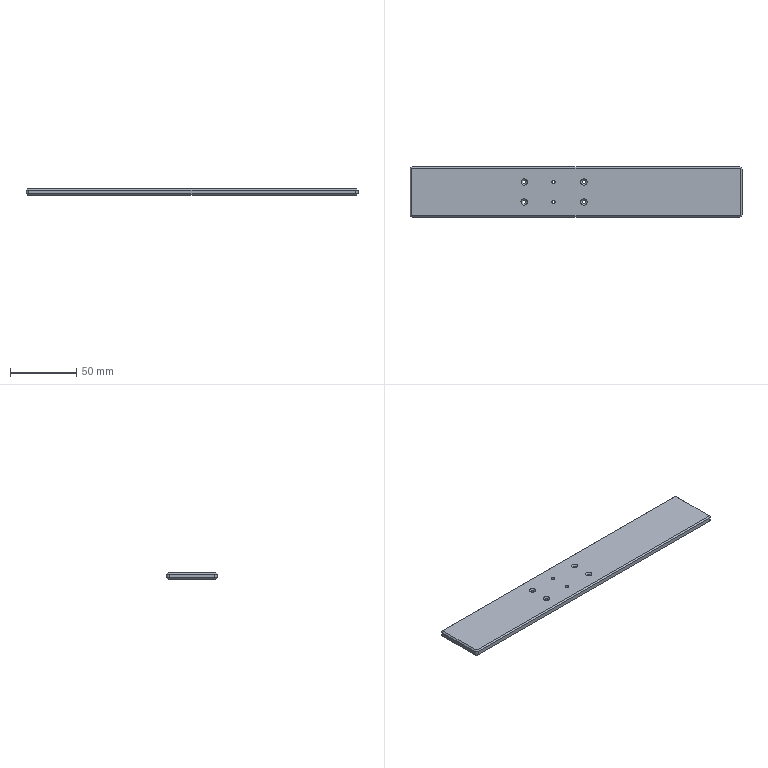NC program | NX | posted with a generic post | part box 250 x 38 x 5 mm
Lines 65 to 892 of 15324:
(ZLEVEL_PROFILE_COPY_COPY_1_COPY_COPY_1_COPY , TOOL : D2)
N128 T08 M6
N130 G54
N132 G17 G0 G90 X-39.808 Y-6.39 S7000 M3
N134 G43 Z35. H8
N136 Z6.5
N138 G94 G1 X-39.937 Y-6.474 Z6.492 F1000.
N140 X-40.219 Y-6.833 Z6.468
N142 X-40.369 Y-7.263 Z6.444
N144 X-40.372 Y-7.72 Z6.42
N146 X-40.227 Y-8.152 Z6.396
N148 X-40.037 Y-8.425 Z6.379
N150 X-39.786 Y-8.646 Z6.361
N152 X-39.49 Y-8.8 Z6.344
N154 X-39.166 Y-8.88 Z6.326
N156 X-38.834 Z6.309
N158 X-38.48 Y-8.789 Z6.29
N160 X-38.162 Y-8.609 Z6.271
N162 X-37.903 Y-8.352 Z6.252
N164 X-37.731 Y-8.067 Z6.234
N166 X-37.616 Y-7.621 Z6.21
N168 X-37.652 Y-7.163 Z6.186
N170 X-37.836 Y-6.741 Z6.162
N172 X-38.148 Y-6.403 Z6.138
N174 X-38.433 Y-6.231 Z6.12
N176 X-38.827 Y-6.121 Z6.099
N178 X-39.235 Y-6.13 Z6.077
N180 X-39.554 Y-6.226 Z6.06
N182 X-39.937 Y-6.474 Z6.036
N184 X-40.219 Y-6.833 Z6.012
N186 X-40.369 Y-7.263 Z5.988
N188 X-40.372 Y-7.72 Z5.964
N190 X-40.227 Y-8.152 Z5.94
N192 X-40.037 Y-8.425 Z5.923
N194 X-39.786 Y-8.646 Z5.905
N196 X-39.49 Y-8.8 Z5.888
N198 X-39.166 Y-8.88 Z5.871
N200 X-38.834 Z5.853
N202 X-38.48 Y-8.789 Z5.834
N204 X-38.162 Y-8.609 Z5.815
N206 X-37.903 Y-8.352 Z5.796
N208 X-37.731 Y-8.067 Z5.778
N210 X-37.616 Y-7.621 Z5.754
N212 X-37.652 Y-7.163 Z5.73
N214 X-37.836 Y-6.741 Z5.706
N216 X-38.148 Y-6.403 Z5.682
N218 X-38.433 Y-6.231 Z5.664
N220 X-38.827 Y-6.121 Z5.643
N222 X-39.235 Y-6.13 Z5.622
N224 X-39.554 Y-6.226 Z5.604
N226 X-39.937 Y-6.474 Z5.58
N228 X-40.219 Y-6.833 Z5.556
N230 X-40.369 Y-7.263 Z5.532
N232 X-40.372 Y-7.72 Z5.508
N234 X-40.227 Y-8.152 Z5.485
N236 X-40.037 Y-8.425 Z5.467
N238 X-39.786 Y-8.646 Z5.45
N240 X-39.49 Y-8.8 Z5.432
N242 X-39.166 Y-8.88 Z5.415
N244 X-38.834 Z5.397
N246 X-38.48 Y-8.789 Z5.378
N248 X-38.162 Y-8.609 Z5.359
N250 X-37.903 Y-8.352 Z5.34
N252 X-37.731 Y-8.067 Z5.322
N254 X-37.616 Y-7.621 Z5.298
N256 X-37.652 Y-7.163 Z5.274
N258 X-37.836 Y-6.741 Z5.25
N260 X-38.148 Y-6.403 Z5.226
N262 X-38.433 Y-6.231 Z5.208
N264 X-38.827 Y-6.121 Z5.187
N266 X-39.235 Y-6.13 Z5.166
N268 X-39.554 Y-6.226 Z5.148
N270 X-39.937 Y-6.474 Z5.124
N272 X-40.219 Y-6.833 Z5.1
N274 X-40.369 Y-7.263 Z5.076
N276 X-40.372 Y-7.72 Z5.053
N278 X-40.227 Y-8.152 Z5.029
N280 X-40.037 Y-8.425 Z5.011
N282 X-39.786 Y-8.646 Z4.994
N284 X-39.49 Y-8.8 Z4.976
N286 X-39.166 Y-8.88 Z4.959
N288 X-39. Z4.95
N290 G3 X-37.621 Y-7.5 R1.379
N292 X-39. Y-8.88 R-1.379
N294 G1 X-38.905 Y-8.875 Z4.948
N296 X-38.81 Y-8.863 Z4.947
N298 X-38.717 Y-8.845 Z4.945
N300 X-38.625 Y-8.821 Z4.943
N302 X-38.535 Y-8.79 Z4.942
N304 X-38.447 Y-8.753 Z4.94
N306 X-38.363 Y-8.71 Z4.938
N308 X-38.282 Y-8.662 Z4.937
N310 X-38.204 Y-8.608 Z4.935
N312 X-38.13 Y-8.549 Z4.933
N314 X-38.061 Y-8.485 Z4.932
N316 X-37.996 Y-8.417 Z4.93
N318 X-37.937 Y-8.344 Z4.928
N320 X-37.882 Y-8.268 Z4.927
N322 X-37.833 Y-8.188 Z4.925
N324 X-37.79 Y-8.105 Z4.923
N326 X-37.752 Y-8.019 Z4.922
N328 X-37.721 Y-7.931 Z4.92
N330 X-37.696 Y-7.841 Z4.918
N332 X-37.677 Y-7.75 Z4.917
N334 X-37.665 Y-7.657 Z4.915
N336 X-37.659 Y-7.564 Z4.913
N338 Y-7.472 Z4.912
N340 X-37.666 Y-7.379 Z4.91
N342 X-37.679 Y-7.288 Z4.908
N344 X-37.699 Y-7.197 Z4.907
N346 X-37.724 Y-7.108 Z4.905
N348 X-37.756 Y-7.021 Z4.903
N350 X-37.794 Y-6.937 Z4.902
N352 X-37.837 Y-6.856 Z4.9
N354 G3 X-39. Y-8.83 R-1.329
N356 G1 X-38.905 Y-8.824 Z4.898
N358 X-38.81 Y-8.813 Z4.897
N360 X-38.717 Y-8.794 Z4.895
N362 X-38.625 Y-8.769 Z4.893
N364 X-38.536 Y-8.737 Z4.892
N366 X-38.449 Y-8.699 Z4.89
N368 X-38.365 Y-8.655 Z4.888
N370 X-38.285 Y-8.605 Z4.887
N372 X-38.208 Y-8.549 Z4.885
N374 X-38.136 Y-8.489 Z4.883
N376 X-38.069 Y-8.423 Z4.882
N378 X-38.006 Y-8.353 Z4.88
N380 X-37.949 Y-8.278 Z4.878
N382 X-37.897 Y-8.2 Z4.877
N384 X-37.851 Y-8.118 Z4.875
N386 X-37.811 Y-8.033 Z4.873
N388 X-37.778 Y-7.946 Z4.872
N390 X-37.75 Y-7.857 Z4.87
N392 X-37.73 Y-7.766 Z4.868
N394 X-37.716 Y-7.674 Z4.867
N396 X-37.708 Y-7.581 Z4.865
N398 X-37.707 Y-7.488 Z4.863
N400 X-37.713 Y-7.396 Z4.862
N402 X-37.726 Y-7.304 Z4.86
N404 X-37.745 Y-7.213 Z4.858
N406 X-37.77 Y-7.124 Z4.857
N408 X-37.802 Y-7.038 Z4.855
N410 X-37.839 Y-6.953 Z4.853
N412 X-37.883 Y-6.872 Z4.852
N414 X-37.932 Y-6.795 Z4.85
N416 G3 X-39. Y-8.78 R-1.279
N418 G1 X-38.905 Y-8.774 Z4.848
N420 X-38.81 Y-8.762 Z4.847
N422 X-38.717 Y-8.743 Z4.845
N424 X-38.626 Y-8.717 Z4.843
N426 X-38.537 Y-8.684 Z4.842
N428 X-38.45 Y-8.644 Z4.84
N430 X-38.368 Y-8.599 Z4.838
N432 X-38.288 Y-8.547 Z4.837
N434 X-38.213 Y-8.49 Z4.835
N436 X-38.143 Y-8.427 Z4.833
N438 X-38.077 Y-8.36 Z4.832
N440 X-38.017 Y-8.287 Z4.83
N442 X-37.962 Y-8.211 Z4.828
N444 X-37.914 Y-8.131 Z4.827
N446 X-37.871 Y-8.047 Z4.825
N448 X-37.835 Y-7.961 Z4.823
N450 X-37.806 Y-7.872 Z4.822
N452 X-37.783 Y-7.782 Z4.82
N454 X-37.767 Y-7.69 Z4.818
N456 X-37.758 Y-7.597 Z4.817
N458 X-37.756 Y-7.505 Z4.815
N460 X-37.76 Y-7.412 Z4.813
N462 X-37.772 Y-7.32 Z4.812
N464 X-37.79 Y-7.229 Z4.81
N466 X-37.816 Y-7.14 Z4.808
N468 X-37.847 Y-7.054 Z4.807
N470 X-37.885 Y-6.97 Z4.805
N472 X-37.929 Y-6.889 Z4.803
N474 X-37.979 Y-6.812 Z4.802
N476 X-38.035 Y-6.738 Z4.8
N478 G3 X-39. Y-8.73 R-1.229
N480 G1 X-38.905 Y-8.724 Z4.798
N482 X-38.81 Y-8.711 Z4.797
N484 X-38.717 Y-8.691 Z4.795
N486 X-38.626 Y-8.664 Z4.793
N488 X-38.538 Y-8.63 Z4.792
N490 X-38.452 Y-8.589 Z4.79
N492 X-38.37 Y-8.542 Z4.788
N494 X-38.292 Y-8.489 Z4.787
N496 X-38.219 Y-8.43 Z4.785
N498 X-38.15 Y-8.365 Z4.783
N500 X-38.087 Y-8.296 Z4.782
N502 X-38.029 Y-8.221 Z4.78
N504 X-37.978 Y-8.143 Z4.778
N506 X-37.932 Y-8.061 Z4.777
N508 X-37.893 Y-7.976 Z4.775
N510 X-37.861 Y-7.888 Z4.773
N512 X-37.836 Y-7.798 Z4.772
N514 X-37.818 Y-7.706 Z4.77
N516 X-37.808 Y-7.614 Z4.768
N518 X-37.804 Y-7.521 Z4.767
N520 X-37.808 Y-7.428 Z4.765
N522 X-37.818 Y-7.336 Z4.763
N524 X-37.836 Y-7.246 Z4.762
N526 X-37.861 Y-7.156 Z4.76
N528 X-37.893 Y-7.07 Z4.758
N530 X-37.931 Y-6.986 Z4.757
N532 X-37.976 Y-6.905 Z4.755
N534 X-38.026 Y-6.829 Z4.753
N536 X-38.082 Y-6.756 Z4.752
N538 X-38.144 Y-6.688 Z4.75
N540 G3 X-39. Y-8.68 R-1.179
N542 G1 X-38.905 Y-8.674 Z4.748
N544 X-38.81 Y-8.661 Z4.747
N546 X-38.718 Y-8.64 Z4.745
N548 X-38.627 Y-8.612 Z4.743
N550 X-38.539 Y-8.577 Z4.742
N552 X-38.454 Y-8.534 Z4.74
N554 X-38.373 Y-8.485 Z4.738
N556 X-38.296 Y-8.43 Z4.737
N558 X-38.225 Y-8.369 Z4.735
N560 X-38.158 Y-8.302 Z4.733
N562 X-38.097 Y-8.231 Z4.732
N564 X-38.043 Y-8.154 Z4.73
N566 X-37.994 Y-8.074 Z4.728
N568 X-37.953 Y-7.99 Z4.727
N570 X-37.918 Y-7.903 Z4.725
N572 X-37.891 Y-7.814 Z4.723
N574 X-37.871 Y-7.723 Z4.722
N576 X-37.858 Y-7.63 Z4.72
N578 X-37.853 Y-7.538 Z4.718
N580 X-37.855 Y-7.445 Z4.717
N582 X-37.865 Y-7.353 Z4.715
N584 X-37.882 Y-7.262 Z4.713
N586 X-37.907 Y-7.173 Z4.712
N588 X-37.938 Y-7.086 Z4.71
N590 X-37.977 Y-7.002 Z4.708
N592 X-38.022 Y-6.922 Z4.707
N594 X-38.073 Y-6.846 Z4.705
N596 X-38.131 Y-6.774 Z4.703
N598 X-38.193 Y-6.707 Z4.702
N600 X-38.261 Y-6.646 Z4.7
N602 G3 X-39. Y-8.63 R-1.129
N604 G1 X-38.905 Y-8.624 Z4.698
N606 X-38.811 Y-8.61 Z4.697
N608 X-38.718 Y-8.589 Z4.695
N610 X-38.628 Y-8.559 Z4.693
N612 X-38.54 Y-8.523 Z4.692
N614 X-38.456 Y-8.479 Z4.69
N616 X-38.377 Y-8.428 Z4.688
N618 X-38.301 Y-8.371 Z4.687
N620 X-38.232 Y-8.307 Z4.685
N622 X-38.167 Y-8.238 Z4.683
N624 X-38.109 Y-8.165 Z4.682
N626 X-38.058 Y-8.086 Z4.68
N628 X-38.013 Y-8.004 Z4.678
N630 X-37.976 Y-7.918 Z4.677
N632 X-37.946 Y-7.829 Z4.675
N634 X-37.923 Y-7.739 Z4.673
N636 X-37.909 Y-7.647 Z4.672
N638 X-37.902 Y-7.554 Z4.67
N640 X-37.903 Y-7.461 Z4.668
N642 X-37.912 Y-7.369 Z4.667
N644 X-37.928 Y-7.278 Z4.665
N646 X-37.952 Y-7.189 Z4.663
N648 X-37.984 Y-7.102 Z4.662
N650 X-38.023 Y-7.018 Z4.66
N652 X-38.068 Y-6.938 Z4.658
N654 X-38.121 Y-6.863 Z4.657
N656 X-38.179 Y-6.792 Z4.655
N658 X-38.243 Y-6.726 Z4.653
N660 X-38.312 Y-6.666 Z4.652
N662 X-38.386 Y-6.612 Z4.65
N664 G3 X-39. Y-8.58 R-1.079
N666 G1 X-38.905 Y-8.574 Z4.648
N668 X-38.811 Y-8.559 Z4.647
N670 X-38.718 Y-8.537 Z4.645
N672 X-38.628 Y-8.506 Z4.643
N674 X-38.542 Y-8.468 Z4.642
N676 X-38.459 Y-8.422 Z4.64
N678 X-38.38 Y-8.37 Z4.638
N680 X-38.307 Y-8.31 Z4.637
N682 X-38.239 Y-8.245 Z4.635
N684 X-38.178 Y-8.173 Z4.633
N686 X-38.123 Y-8.097 Z4.632
N688 X-38.075 Y-8.017 Z4.63
N690 X-38.035 Y-7.932 Z4.628
N692 X-38.002 Y-7.845 Z4.627
N694 X-37.977 Y-7.755 Z4.625
N696 X-37.96 Y-7.663 Z4.623
N698 X-37.951 Y-7.571 Z4.622
N700 Y-7.478 Z4.62
N702 X-37.958 Y-7.385 Z4.618
N704 X-37.974 Y-7.294 Z4.617
N706 X-37.998 Y-7.205 Z4.615
N708 X-38.03 Y-7.118 Z4.613
N710 X-38.069 Y-7.035 Z4.612
N712 X-38.115 Y-6.955 Z4.61
N714 X-38.168 Y-6.88 Z4.608
N716 X-38.227 Y-6.81 Z4.607
N718 X-38.292 Y-6.746 Z4.605
N720 X-38.363 Y-6.687 Z4.603
N722 X-38.438 Y-6.636 Z4.602
N724 X-38.517 Y-6.591 Z4.6
N726 G3 X-39. Y-8.53 R-1.029
N728 G1 X-38.905 Y-8.523 Z4.598
N730 X-38.811 Y-8.509 Z4.597
N732 X-38.706 Y-8.481 Z4.595
N734 X-38.629 Y-8.453 Z4.593
N736 X-38.529 Y-8.406 Z4.591
N738 X-38.461 Y-8.366 Z4.59
N740 X-38.372 Y-8.301 Z4.588
N742 X-38.313 Y-8.249 Z4.587
N744 X-38.238 Y-8.169 Z4.585
N746 X-38.19 Y-8.108 Z4.583
N748 X-38.13 Y-8.015 Z4.581
N750 X-38.094 Y-7.946 Z4.58
N752 X-38.053 Y-7.845 Z4.578
N754 X-38.031 Y-7.771 Z4.577
N756 X-38.009 Y-7.664 Z4.575
N758 X-38.001 Y-7.587 Z4.573
N760 X-37.999 Y-7.478 Z4.571
N762 X-38.005 Y-7.402 Z4.57
N764 X-38.024 Y-7.295 Z4.568
N766 X-38.044 Y-7.221 Z4.567
N768 X-38.081 Y-7.12 Z4.565
N770 X-38.115 Y-7.051 Z4.563
N772 X-38.17 Y-6.958 Z4.561
N774 X-38.215 Y-6.897 Z4.56
N776 X-38.287 Y-6.817 Z4.558
N778 X-38.342 Y-6.765 Z4.557
N780 X-38.427 Y-6.7 Z4.555
N782 X-38.491 Y-6.659 Z4.553
N784 X-38.571 Y-6.617 Z4.552
N786 X-38.656 Y-6.583 Z4.55
N788 G3 X-39. Y-8.48 R-0.979
N790 G1 X-38.905 Y-8.473 Z4.548
N792 X-38.811 Y-8.458 Z4.547
N794 X-38.706 Y-8.429 Z4.545
N796 X-38.63 Y-8.4 Z4.543
N798 X-38.532 Y-8.35 Z4.541
N800 X-38.465 Y-8.308 Z4.54
N802 X-38.378 Y-8.241 Z4.538
N804 X-38.321 Y-8.187 Z4.537
N806 X-38.248 Y-8.104 Z4.535
N808 X-38.203 Y-8.04 Z4.533
N810 X-38.149 Y-7.945 Z4.531
N812 X-38.117 Y-7.875 Z4.53
N814 X-38.082 Y-7.771 Z4.528
N816 X-38.064 Y-7.696 Z4.527
N818 X-38.05 Y-7.588 Z4.525
N820 X-38.047 Y-7.511 Z4.523
N822 X-38.054 Y-7.402 Z4.521
N824 X-38.067 Y-7.326 Z4.52
N826 X-38.094 Y-7.222 Z4.518
N828 X-38.121 Y-7.15 Z4.517
N830 X-38.168 Y-7.053 Z4.515
N832 X-38.208 Y-6.988 Z4.513
N834 X-38.273 Y-6.903 Z4.511
N836 X-38.325 Y-6.847 Z4.51
N838 X-38.405 Y-6.776 Z4.508
N840 X-38.466 Y-6.731 Z4.507
N842 X-38.558 Y-6.677 Z4.505
N844 X-38.626 Y-6.645 Z4.503
N846 X-38.712 Y-6.615 Z4.502
N848 X-38.8 Y-6.592 Z4.5
N850 G3 X-39. Y-8.43 R-0.929
N852 G1 X-38.88 Y-8.42 Z4.498
N854 X-38.811 Y-8.407 Z4.497
N856 X-38.703 Y-8.375 Z4.495
N858 X-38.631 Y-8.346 Z4.493
N860 X-38.533 Y-8.294 Z4.491
N862 X-38.468 Y-8.25 Z4.49
N864 X-38.384 Y-8.18 Z4.488
N866 X-38.329 Y-8.124 Z4.487
N868 X-38.261 Y-8.038 Z4.485
N870 X-38.219 Y-7.972 Z4.483
N872 X-38.17 Y-7.874 Z4.481
N874 X-38.142 Y-7.802 Z4.48
N876 X-38.114 Y-7.696 Z4.478
N878 X-38.102 Y-7.62 Z4.477
N880 X-38.096 Y-7.511 Z4.475
N882 X-38.1 Y-7.434 Z4.473
N884 X-38.116 Y-7.327 Z4.471
N886 X-38.135 Y-7.253 Z4.47
N888 X-38.173 Y-7.152 Z4.468
N890 X-38.207 Y-7.083 Z4.467
N892 X-38.264 Y-6.992 Z4.465
N894 X-38.311 Y-6.932 Z4.463
N896 X-38.385 Y-6.855 Z4.461
N898 X-38.443 Y-6.806 Z4.46
N900 X-38.532 Y-6.746 Z4.458
N902 X-38.598 Y-6.71 Z4.457
N904 X-38.696 Y-6.67 Z4.455
N906 X-38.769 Y-6.648 Z4.453
N908 X-38.857 Y-6.63 Z4.452
N910 X-38.947 Y-6.622 Z4.45
N912 G3 X-39. Y-8.38 R-0.879
N914 G1 X-38.88 Y-8.369 Z4.448
N916 X-38.811 Y-8.356 Z4.447
N918 X-38.704 Y-8.322 Z4.445
N920 X-38.633 Y-8.292 Z4.443
N922 X-38.536 Y-8.237 Z4.441
N924 X-38.473 Y-8.191 Z4.44
N926 X-38.391 Y-8.118 Z4.438
N928 X-38.339 Y-8.06 Z4.437
N930 X-38.275 Y-7.97 Z4.435
N932 X-38.237 Y-7.902 Z4.433
N934 X-38.194 Y-7.802 Z4.431
N936 X-38.171 Y-7.728 Z4.43
N938 X-38.151 Y-7.621 Z4.428
N940 X-38.145 Y-7.544 Z4.427
N942 X-38.148 Y-7.435 Z4.425
N944 X-38.159 Y-7.359 Z4.423
N946 X-38.185 Y-7.254 Z4.421
N948 X-38.212 Y-7.182 Z4.42
N950 X-38.26 Y-7.086 Z4.418
N952 X-38.302 Y-7.022 Z4.417
N954 X-38.37 Y-6.939 Z4.415
N956 X-38.424 Y-6.885 Z4.413
N958 X-38.507 Y-6.819 Z4.411
N960 X-38.571 Y-6.778 Z4.41
N962 X-38.667 Y-6.732 Z4.408
N964 X-38.738 Y-6.706 Z4.407
N966 X-38.841 Y-6.681 Z4.405
N968 X-38.915 Y-6.671 Z4.403
N970 X-39.005 Y-6.669 Z4.402
N972 X-39.095 Y-6.676 Z4.4
N974 G3 X-39. Y-8.33 R0.829
N976 G1 X-38.88 Y-8.319 Z4.398
N978 X-38.811 Y-8.304 Z4.397
N980 X-38.704 Y-8.269 Z4.395
N982 X-38.634 Y-8.237 Z4.393
N984 X-38.54 Y-8.18 Z4.391
N986 X-38.478 Y-8.132 Z4.39
N988 X-38.399 Y-8.055 Z4.388
N990 X-38.35 Y-7.994 Z4.387
N992 X-38.291 Y-7.901 Z4.385
N994 X-38.258 Y-7.831 Z4.383
N996 X-38.222 Y-7.728 Z4.381
N998 X-38.205 Y-7.652 Z4.38
N1000 X-38.194 Y-7.544 Z4.378
N1002 X-38.195 Y-7.467 Z4.377
N1004 X-38.208 Y-7.36 Z4.375
N1006 X-38.226 Y-7.285 Z4.373
N1008 X-38.264 Y-7.184 Z4.371
N1010 X-38.299 Y-7.116 Z4.37
N1012 X-38.358 Y-7.026 Z4.368
N1014 X-38.407 Y-6.968 Z4.367
N1016 X-38.485 Y-6.895 Z4.365
N1018 X-38.546 Y-6.85 Z4.363
N1020 X-38.639 Y-6.797 Z4.361
N1022 X-38.708 Y-6.767 Z4.36
N1024 X-38.81 Y-6.736 Z4.358
N1026 X-38.883 Y-6.723 Z4.357
N1028 X-38.989 Y-6.716 Z4.355
N1030 X-39.064 Y-6.72 Z4.353
N1032 X-39.152 Y-6.734 Z4.352
N1034 X-39.239 Y-6.758 Z4.35
N1036 G3 X-39. Y-8.28 R0.779
N1038 G1 X-38.879 Y-8.268 Z4.348
N1040 X-38.812 Y-8.253 Z4.347
N1042 X-38.705 Y-8.216 Z4.345
N1044 X-38.636 Y-8.182 Z4.343
N1046 X-38.544 Y-8.121 Z4.341
N1048 X-38.484 Y-8.071 Z4.34
N1050 X-38.409 Y-7.99 Z4.338
N1052 X-38.364 Y-7.927 Z4.337
N1054 X-38.311 Y-7.831 Z4.335
N1056 X-38.282 Y-7.759 Z4.333
N1058 X-38.255 Y-7.653 Z4.331
N1060 X-38.244 Y-7.576 Z4.33
N1062 X-38.243 Y-7.468 Z4.328
N1064 X-38.252 Y-7.391 Z4.327
N1066 X-38.277 Y-7.286 Z4.325
N1068 X-38.303 Y-7.214 Z4.323
N1070 X-38.353 Y-7.119 Z4.321
N1072 X-38.396 Y-7.056 Z4.32
N1074 X-38.467 Y-6.976 Z4.318
N1076 X-38.524 Y-6.925 Z4.317
N1078 X-38.612 Y-6.865 Z4.315
N1080 X-38.679 Y-6.83 Z4.313
N1082 X-38.779 Y-6.793 Z4.311
N1084 X-38.852 Y-6.776 Z4.31
N1086 X-38.957 Y-6.764 Z4.308
N1088 X-39.032 Y-6.765 Z4.307
N1090 X-39.136 Y-6.779 Z4.305
N1092 X-39.208 Y-6.797 Z4.303
N1094 X-39.292 Y-6.83 Z4.302
N1096 X-39.371 Y-6.872 Z4.3
N1098 G3 X-39. Y-8.23 R0.729
N1100 G1 X-38.879 Y-8.217 Z4.298
N1102 X-38.812 Y-8.201 Z4.297
N1104 X-38.707 Y-8.162 Z4.295
N1106 X-38.639 Y-8.126 Z4.293
N1108 X-38.548 Y-8.062 Z4.291
N1110 X-38.491 Y-8.009 Z4.29
N1112 X-38.421 Y-7.924 Z4.288
N1114 X-38.38 Y-7.858 Z4.287
N1116 X-38.334 Y-7.759 Z4.285
N1118 X-38.311 Y-7.685 Z4.283
N1120 X-38.293 Y-7.577 Z4.281
N1122 X-38.291 Y-7.5 Z4.28
N1124 X-38.301 Y-7.392 Z4.278
N1126 X-38.318 Y-7.317 Z4.277
N1128 X-38.355 Y-7.216 Z4.275
N1130 X-38.391 Y-7.149 Z4.273
N1132 X-38.453 Y-7.061 Z4.271
N1134 X-38.505 Y-7.005 Z4.27
N1136 X-38.588 Y-6.937 Z4.268
N1138 X-38.652 Y-6.897 Z4.267
N1140 X-38.748 Y-6.853 Z4.265
N1142 X-38.821 Y-6.831 Z4.263
N1144 X-38.925 Y-6.813 Z4.261
N1146 X-39. Y-6.811 Z4.26
N1148 X-39.105 Y-6.82 Z4.258
N1150 X-39.177 Y-6.837 Z4.257
N1152 X-39.276 Y-6.874 Z4.255
N1154 X-39.341 Y-6.909 Z4.253
N1156 X-39.414 Y-6.959 Z4.252
N1158 X-39.48 Y-7.019 Z4.25
N1160 G3 X-39. Y-8.18 R0.679
N1162 G1 X-38.879 Y-8.166 Z4.248
N1164 X-38.812 Y-8.15 Z4.247
N1166 X-38.708 Y-8.108 Z4.245
N1168 X-38.641 Y-8.069 Z4.243
N1170 X-38.554 Y-8.001 Z4.241
N1172 X-38.5 Y-7.945 Z4.24
N1174 X-38.436 Y-7.856 Z4.238
N1176 X-38.399 Y-7.788 Z4.237
N1178 X-38.362 Y-7.685 Z4.235
N1180 X-38.346 Y-7.609 Z4.233
N1182 X-38.339 Y-7.501 Z4.231
N1184 X-38.345 Y-7.424 Z4.23
N1186 X-38.368 Y-7.318 Z4.228
N1188 X-38.395 Y-7.247 Z4.227
N1190 X-38.446 Y-7.152 Z4.225
N1192 X-38.491 Y-7.091 Z4.223
N1194 X-38.566 Y-7.015 Z4.221
N1196 X-38.627 Y-6.968 Z4.22
N1198 X-38.72 Y-6.916 Z4.218
N1200 X-38.79 Y-6.889 Z4.217
N1202 X-38.893 Y-6.865 Z4.215
N1204 X-38.968 Y-6.858 Z4.213
N1206 X-39.073 Y-6.863 Z4.211
N1208 X-39.146 Y-6.877 Z4.21
N1210 X-39.245 Y-6.912 Z4.208
N1212 X-39.312 Y-6.945 Z4.207
N1214 X-39.397 Y-7.005 Z4.205
N1216 X-39.451 Y-7.056 Z4.203
N1218 X-39.507 Y-7.124 Z4.202
N1220 X-39.553 Y-7.2 Z4.2
N1222 G3 X-39. Y-8.13 R0.629
N1224 G1 X-38.876 Y-8.115 Z4.198
N1226 X-38.809 Y-8.096 Z4.196
N1228 X-38.704 Y-8.049 Z4.194
N1230 X-38.639 Y-8.007 Z4.193
N1232 X-38.554 Y-7.932 Z4.191
N1234 X-38.504 Y-7.87 Z4.189
N1236 X-38.447 Y-7.774 Z4.187
N1238 X-38.418 Y-7.7 Z4.186
N1240 X-38.394 Y-7.592 Z4.184
N1242 X-38.388 Y-7.513 Z4.182
N1244 X-38.398 Y-7.403 Z4.18
N1246 X-38.417 Y-7.327 Z4.179
N1248 X-38.46 Y-7.226 Z4.176
N1250 X-38.5 Y-7.16 Z4.175
N1252 X-38.571 Y-7.077 Z4.173
N1254 X-38.63 Y-7.026 Z4.171
N1256 X-38.723 Y-6.969 Z4.169
N1258 X-38.794 Y-6.939 Z4.168
N1260 X-38.898 Y-6.913 Z4.166
N1262 X-38.975 Y-6.907 Z4.164
N1264 X-39.081 Y-6.914 Z4.162
N1266 X-39.156 Y-6.931 Z4.161
N1268 X-39.255 Y-6.97 Z4.159
N1270 X-39.32 Y-7.008 Z4.157
N1272 X-39.402 Y-7.075 Z4.155
N1274 X-39.452 Y-7.131 Z4.154
N1276 X-39.502 Y-7.206 Z4.152
N1278 X-39.539 Y-7.288 Z4.15
N1280 G3 X-39. Y-8.08 R0.579
N1282 G1 X-38.879 Y-8.064 Z4.148
N1284 X-38.813 Y-8.044 Z4.146
N1286 X-38.711 Y-7.995 Z4.144
N1288 X-38.648 Y-7.951 Z4.142
N1290 X-38.57 Y-7.873 Z4.14
N1292 X-38.524 Y-7.81 Z4.138
N1294 X-38.475 Y-7.712 Z4.136
N1296 X-38.453 Y-7.637 Z4.135
N1298 X-38.439 Y-7.529 Z4.132
N1300 X-38.442 Y-7.452 Z4.131
N1302 X-38.464 Y-7.346 Z4.129
N1304 X-38.491 Y-7.275 Z4.127
N1306 X-38.546 Y-7.183 Z4.125
N1308 X-38.595 Y-7.124 Z4.123
N1310 X-38.676 Y-7.055 Z4.121
N1312 X-38.741 Y-7.016 Z4.119
N1314 X-38.839 Y-6.978 Z4.117
N1316 X-38.913 Y-6.962 Z4.115
N1318 X-39.018 Y-6.958 Z4.113
N1320 X-39.092 Y-6.967 Z4.112
N1322 X-39.192 Y-6.997 Z4.109
N1324 X-39.258 Y-7.029 Z4.108
N1326 X-39.343 Y-7.089 Z4.105
N1328 X-39.395 Y-7.141 Z4.104
N1330 X-39.447 Y-7.212 Z4.102
N1332 X-39.486 Y-7.291 Z4.1
N1334 G3 X-39. Y-8.03 R0.529
N1336 G1 X-38.881 Y-8.013 Z4.097
N1338 X-38.817 Y-7.992 Z4.096
N1340 X-38.719 Y-7.941 Z4.093
N1342 X-38.66 Y-7.895 Z4.092
N1344 X-38.587 Y-7.814 Z4.089
N1346 X-38.547 Y-7.75 Z4.088
N1348 X-38.508 Y-7.65 Z4.085
N1350 X-38.493 Y-7.576 Z4.083
N1352 X-38.49 Y-7.47 Z4.081
N1354 X-38.502 Y-7.395 Z4.079
N1356 X-38.537 Y-7.296 Z4.077
N1358 X-38.573 Y-7.231 Z4.075
N1360 X-38.64 Y-7.15 Z4.073
N1362 X-38.696 Y-7.102 Z4.071
N1364 X-38.786 Y-7.051 Z4.068
N1366 X-38.855 Y-7.026 Z4.067
N1368 X-38.956 Y-7.008 Z4.064
N1370 X-39.029 Y-7.009 Z4.063
N1372 X-39.129 Y-7.028 Z4.06
N1374 X-39.197 Y-7.053 Z4.058
N1376 X-39.283 Y-7.106 Z4.056
N1378 X-39.337 Y-7.153 Z4.054
N1380 X-39.391 Y-7.219 Z4.052
N1382 X-39.433 Y-7.294 Z4.05
N1384 G3 X-39. Y-7.98 R0.479
N1386 G1 X-38.885 Y-7.962 Z4.047
N1388 X-38.822 Y-7.94 Z4.045
N1390 X-38.729 Y-7.887 Z4.043
N1392 X-38.673 Y-7.839 Z4.041
N1394 X-38.608 Y-7.756 Z4.038
N1396 X-38.575 Y-7.69 Z4.036
N1398 X-38.546 Y-7.59 Z4.034
N1400 X-38.539 Y-7.517 Z4.032
N1402 X-38.549 Y-7.414 Z4.029
N1404 X-38.571 Y-7.344 Z4.027
N1406 X-38.618 Y-7.254 Z4.025
N1408 X-38.663 Y-7.198 Z4.023
N1410 X-38.741 Y-7.133 Z4.02
N1412 X-38.803 Y-7.098 Z4.018
N1414 X-38.898 Y-7.067 Z4.016
N1416 X-38.968 Y-7.058 Z4.014
N1418 X-39.067 Y-7.065 Z4.011
N1420 X-39.135 Y-7.083 Z4.009
N1422 X-39.223 Y-7.125 Z4.006
N1424 X-39.278 Y-7.167 Z4.005
N1426 X-39.335 Y-7.227 Z4.002
N1428 X-39.379 Y-7.297 Z4.
N1430 G3 X-39. Y-7.93 R0.429
N1432 G1 X-38.916 Y-7.919 Z3.998
N1434 X-38.876 Y-7.908 Z3.996
N1436 X-38.854 Y-7.899
N1438 X-38.811 Y-7.879 Z3.994
N1440 X-38.744 Y-7.835 Z3.992
N1442 X-38.714 Y-7.809 Z3.991
N1444 X-38.697 Y-7.791 Z3.99
N1446 X-38.666 Y-7.752 Z3.989
N1448 X-38.626 Y-7.683 Z3.987
N1450 X-38.612 Y-7.647 Z3.986
N1452 X-38.605 Y-7.624 Z3.985
N1454 X-38.594 Y-7.575 Z3.983
N1456 X-38.589 Y-7.497 Z3.981
N1458 X-38.593 Y-7.459 Z3.98
N1460 X-38.596 Y-7.435 Z3.979
N1462 X-38.609 Y-7.388 Z3.978
N1464 X-38.639 Y-7.317 Z3.976
N1466 X-38.658 Y-7.285 Z3.974
N1468 X-38.672 Y-7.265
N1470 X-38.704 Y-7.228 Z3.972
N1472 X-38.762 Y-7.179 Z3.97
N1474 X-38.793 Y-7.16 Z3.969
N1476 X-38.814 Y-7.148 Z3.968
N1478 X-38.858 Y-7.13 Z3.967
N1480 X-38.931 Y-7.112 Z3.964
N1482 X-38.967 Y-7.109 Z3.963
N1484 X-38.991 Y-7.108
N1486 X-39.038 Y-7.111 Z3.961
N1488 X-39.11 Y-7.127 Z3.959
N1490 X-39.143 Y-7.14 Z3.958
N1492 X-39.164 Y-7.15 Z3.957
N1494 X-39.204 Y-7.174 Z3.956
N1496 X-39.24 Y-7.2 Z3.954
N1498 X-39.271 Y-7.231 Z3.953
N1500 X-39.299 Y-7.265 Z3.951
N1502 X-39.324 Y-7.302 Z3.95
N1504 G3 X-39. Y-7.88 R0.379
N1506 G1 X-38.918 Y-7.868 Z3.947
N1508 X-38.88 Y-7.856 Z3.946
N1510 X-38.858 Y-7.847 Z3.945
N1512 X-38.817 Y-7.825 Z3.944
N1514 X-38.755 Y-7.778 Z3.941
N1516 X-38.729 Y-7.751 Z3.94
N1518 X-38.713 Y-7.732 Z3.939
N1520 X-38.687 Y-7.691 Z3.938
N1522 X-38.656 Y-7.621 Z3.935
N1524 X-38.647 Y-7.585 Z3.934
N1526 X-38.643 Y-7.561 Z3.933
N1528 X-38.639 Y-7.513 Z3.931
N1530 X-38.647 Y-7.438 Z3.929
N1532 X-38.657 Y-7.403 Z3.927
N1534 X-38.664 Y-7.381
N1536 X-38.685 Y-7.338 Z3.925
N1538 X-38.727 Y-7.277 Z3.922
N1540 X-38.752 Y-7.252 Z3.921
N1542 X-38.77 Y-7.236 Z3.92
N1544 X-38.808 Y-7.21 Z3.919
N1546 X-38.873 Y-7.178 Z3.916
N1548 X-38.907 Y-7.168 Z3.915
N1550 X-38.93 Y-7.164 Z3.914
N1552 X-38.975 Y-7.159 Z3.913
N1554 X-39.046 Y-7.164 Z3.91
N1556 X-39.08 Y-7.171 Z3.909
N1558 X-39.101 Y-7.178 Z3.908
N1560 X-39.143 Y-7.196 Z3.906
N1562 X-39.179 Y-7.218 Z3.905
N1564 X-39.212 Y-7.244 Z3.903
N1566 X-39.242 Y-7.274 Z3.902
N1568 X-39.268 Y-7.308 Z3.9
N1570 G3 X-39. Y-7.83 R0.329
N1572 G1 X-38.921 Y-7.817 Z3.897
N1574 X-38.885 Y-7.804 Z3.895
N1576 X-38.864 Y-7.794
N1578 X-38.826 Y-7.771 Z3.893
N1580 X-38.769 Y-7.721 Z3.89
N1582 X-38.747 Y-7.692 Z3.889
N1584 X-38.734 Y-7.673 Z3.888
N1586 X-38.713 Y-7.631 Z3.886
N1588 X-38.694 Y-7.56 Z3.883
N1590 X-38.69 Y-7.525 Z3.881
N1592 Y-7.502 Z3.88
N1594 X-38.695 Y-7.456 Z3.879
N1596 X-38.716 Y-7.388 Z3.876
N1598 X-38.732 Y-7.357 Z3.874
N1600 X-38.744 Y-7.338 Z3.873
N1602 X-38.772 Y-7.303 Z3.871
N1604 X-38.826 Y-7.258 Z3.869
N1606 X-38.855 Y-7.241 Z3.867
N1608 X-38.875 Y-7.232 Z3.866
N1610 X-38.917 Y-7.218 Z3.864
N1612 X-38.985 Y-7.21 Z3.861
N1614 X-39.018 Y-7.211 Z3.86
N1616 X-39.039 Y-7.214 Z3.859
N1618 X-39.081 Y-7.225 Z3.857
N1620 X-39.118 Y-7.241 Z3.855
N1622 X-39.152 Y-7.261 Z3.854
N1624 X-39.183 Y-7.286 Z3.852
N1626 X-39.211 Y-7.317 Z3.85
N1628 G3 X-39. Y-7.78 R0.279
N1630 G1 X-38.925 Y-7.766 Z3.847
N1632 X-38.891 Y-7.752 Z3.845
N1634 X-38.872 Y-7.742 Z3.844
N1636 X-38.837 Y-7.717 Z3.842
N1638 X-38.789 Y-7.664 Z3.838
N1640 X-38.771 Y-7.635 Z3.837
N1642 X-38.761 Y-7.615 Z3.836
N1644 X-38.747 Y-7.573 Z3.833
N1646 X-38.741 Y-7.504 Z3.83
N1648 X-38.744 Y-7.471 Z3.828
N1650 X-38.748 Y-7.45 Z3.827
N1652 X-38.762 Y-7.409 Z3.825
N1654 X-38.797 Y-7.352 Z3.822
N1656 X-38.818 Y-7.329 Z3.82
N1658 X-38.834 Y-7.315 Z3.819
N1660 X-38.869 Y-7.292 Z3.817
N1662 X-38.929 Y-7.268 Z3.813
N1664 X-38.959 Y-7.262 Z3.812
N1666 X-38.979 Y-7.261 Z3.811
N1668 X-39.02 Y-7.263 Z3.808
N1670 X-39.056 Y-7.271 Z3.806
N1672 X-39.091 Y-7.285 Z3.804
N1674 X-39.123 Y-7.304 Z3.802
N1676 X-39.153 Y-7.329 Z3.8
N1678 G3 X-39. Y-7.73 R0.229
N1680 G1 X-38.92 Y-7.715 Z3.796
N1682 X-38.886 Y-7.699 Z3.795
N1684 X-38.869 Y-7.688 Z3.794
N1686 X-38.838 Y-7.662 Z3.792
N1688 X-38.794 Y-7.601 Z3.788
N1690 X-38.781 Y-7.568 Z3.787
N1692 X-38.775 Y-7.546 Z3.786
N1694 X-38.771 Y-7.5 Z3.783
N1696 X-38.783 Y-7.426 Z3.78
N1698 X-38.796 Y-7.394 Z3.778
N1700 X-38.808 Y-7.374 Z3.777
N1702 X-38.838 Y-7.338 Z3.775
N1704 X-38.898 Y-7.294 Z3.772
N1706 X-38.931 Y-7.281 Z3.77
N1708 X-38.953 Y-7.275 Z3.769
N1710 X-39. Y-7.271 Z3.767
N1712 X-39.073 Y-7.283 Z3.763
N1714 X-39.106 Y-7.296 Z3.762
N1716 X-39.126 Y-7.308 Z3.761
N1718 X-39.162 Y-7.338 Z3.758
N1720 X-39.191 Y-7.373 Z3.756
N1722 X-39.212 Y-7.412 Z3.754
N1724 X-39.225 Y-7.454 Z3.752
N1726 X-39.23 Y-7.5 Z3.75
N1728 G3 X-39. Y-7.73 R0.229
N1730 G1 X-38.92 Y-7.715 Z3.746
N1732 X-38.886 Y-7.699 Z3.745
N1734 X-38.869 Y-7.688 Z3.744
N1736 X-38.838 Y-7.662 Z3.742
N1738 X-38.794 Y-7.601 Z3.738
N1740 X-38.781 Y-7.568 Z3.737
N1742 X-38.775 Y-7.546 Z3.736
N1744 X-38.771 Y-7.5 Z3.733
N1746 X-38.783 Y-7.426 Z3.73
N1748 X-38.796 Y-7.394 Z3.728
N1750 X-38.808 Y-7.374 Z3.727
N1752 X-38.838 Y-7.338 Z3.725
N1754 X-38.898 Y-7.294 Z3.722
N1756 X-38.931 Y-7.281 Z3.72
N1758 X-38.953 Y-7.275 Z3.719
N1760 X-39. Y-7.271 Z3.717
N1762 X-39.073 Y-7.283 Z3.713
N1764 X-39.106 Y-7.296 Z3.712
N1766 X-39.126 Y-7.308 Z3.711
N1768 X-39.162 Y-7.338 Z3.708
N1770 X-39.191 Y-7.373 Z3.706
N1772 X-39.212 Y-7.412 Z3.704
N1774 X-39.225 Y-7.454 Z3.702
N1776 X-39.23 Y-7.5 Z3.7